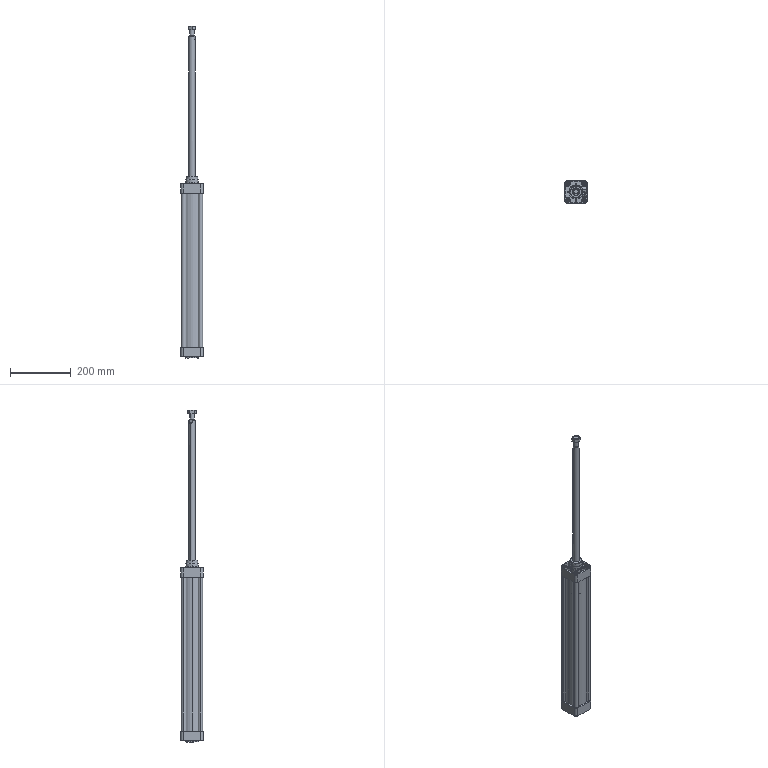Part | SolidWorks | 3 solids | 572 faces | box 75 x 75 x 1095 mm | volume 1179276 mm3 | cylinder 253 | plane 245 | cone 54 | spline 20 | commonest cylinder face diameters 3 x100 19 x20 14 x18 6.647 x16 13 x16 46 x16